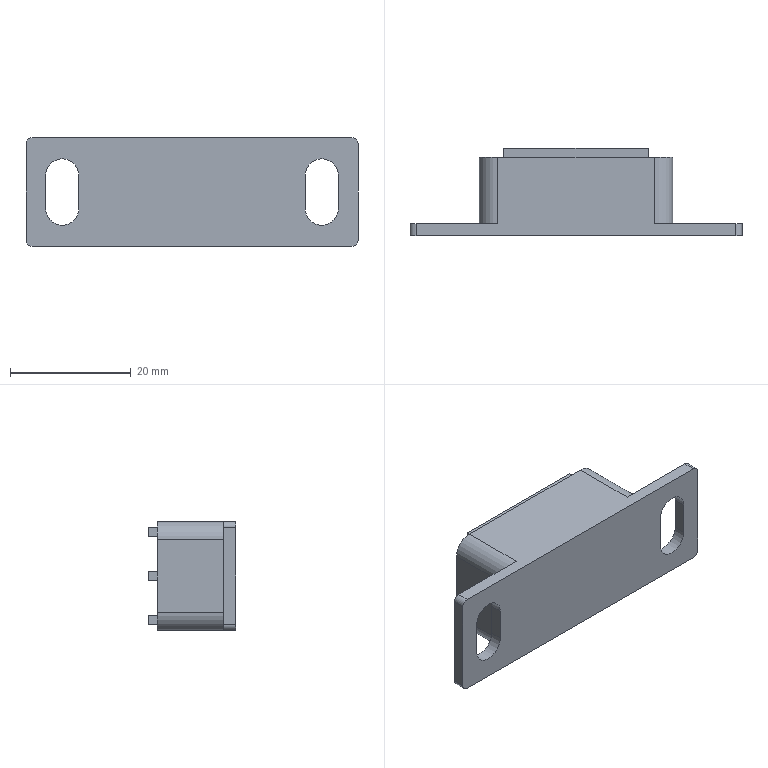Part | SolidWorks | features BaseBody 1 | 1 solid | 43 faces | box 55 x 14.5 x 18 mm | volume 8175 mm3 | plane 29 | cylinder 14 | commonest cylinder face diameters 5.5 x6 2 x4 6 x4
STEP:
#1=CARTESIAN_POINT('',(-18.75,0.,-6.25));
#2=VERTEX_POINT('',#1);
#3=CARTESIAN_POINT('',(-21.5,0.,-3.5));
#4=VERTEX_POINT('',#3);
#5=CARTESIAN_POINT('',(-21.5,0.,-6.25));
#6=DIRECTION('',(0.,-1.,0.));
#7=DIRECTION('',(0.,0.,1.));
#8=AXIS2_PLACEMENT_3D('',#5,#6,#7);
#9=CIRCLE('',#8,2.75);
#10=EDGE_CURVE('',#2,#4,#9,.T.);
#11=ORIENTED_EDGE('',*,*,#10,.T.);
#12=CARTESIAN_POINT('',(-21.5,2.,-3.5));
#13=VERTEX_POINT('',#12);
#14=CARTESIAN_POINT('',(-21.5,2.,-3.5));
#15=DIRECTION('',(0.,1.,0.));
#16=VECTOR('',#15,1000.);
#17=LINE('',#14,#16);
#18=EDGE_CURVE('',#4,#13,#17,.T.);
#19=ORIENTED_EDGE('',*,*,#18,.T.);
#20=CARTESIAN_POINT('',(-18.75,2.,-6.25));
#21=VERTEX_POINT('',#20);
#22=CARTESIAN_POINT('',(-21.5,2.,-6.25));
#23=DIRECTION('',(0.,-1.,0.));
#24=DIRECTION('',(0.,0.,1.));
#25=AXIS2_PLACEMENT_3D('',#22,#23,#24);
#26=CIRCLE('',#25,2.75);
#27=EDGE_CURVE('',#21,#13,#26,.T.);
#28=ORIENTED_EDGE('',*,*,#27,.F.);
#29=CARTESIAN_POINT('',(-18.75,2.,-6.25));
#30=DIRECTION('',(0.,1.,0.));
#31=VECTOR('',#30,1000.);
#32=LINE('',#29,#31);
#33=EDGE_CURVE('',#2,#21,#32,.T.);
#34=ORIENTED_EDGE('',*,*,#33,.F.);
#35=EDGE_LOOP('',(#11,#19,#28,#34));
#36=FACE_OUTER_BOUND('',#35,.T.);
#37=CARTESIAN_POINT('',(-21.5,2.,-6.25));
#38=DIRECTION('',(0.,1.,0.));
#39=DIRECTION('',(0.,0.,1.));
#40=AXIS2_PLACEMENT_3D('',#37,#38,#39);
#41=CYLINDRICAL_SURFACE('',#40,2.75);
#42=ADVANCED_FACE('',(#36),#41,.F.);
#43=CARTESIAN_POINT('',(24.25,0.,-6.25));
#44=VERTEX_POINT('',#43);
#45=CARTESIAN_POINT('',(21.5,0.,-3.5));
#46=VERTEX_POINT('',#45);
#47=CARTESIAN_POINT('',(21.5,0.,-6.25));
#48=DIRECTION('',(0.,-1.,0.));
#49=DIRECTION('',(0.,0.,1.));
#50=AXIS2_PLACEMENT_3D('',#47,#48,#49);
#51=CIRCLE('',#50,2.75);
#52=EDGE_CURVE('',#44,#46,#51,.T.);
#53=ORIENTED_EDGE('',*,*,#52,.T.);
#54=CARTESIAN_POINT('',(21.5,2.,-3.5));
#55=VERTEX_POINT('',#54);
#56=CARTESIAN_POINT('',(21.5,2.,-3.5));
#57=DIRECTION('',(0.,1.,0.));
#58=VECTOR('',#57,1000.);
#59=LINE('',#56,#58);
#60=EDGE_CURVE('',#46,#55,#59,.T.);
#61=ORIENTED_EDGE('',*,*,#60,.T.);
#62=CARTESIAN_POINT('',(24.25,2.,-6.25));
#63=VERTEX_POINT('',#62);
#64=CARTESIAN_POINT('',(21.5,2.,-6.25));
#65=DIRECTION('',(0.,-1.,0.));
#66=DIRECTION('',(0.,0.,1.));
#67=AXIS2_PLACEMENT_3D('',#64,#65,#66);
#68=CIRCLE('',#67,2.75);
#69=EDGE_CURVE('',#63,#55,#68,.T.);
#70=ORIENTED_EDGE('',*,*,#69,.F.);
#71=CARTESIAN_POINT('',(24.25,2.,-6.25));
#72=DIRECTION('',(0.,1.,0.));
#73=VECTOR('',#72,1000.);
#74=LINE('',#71,#73);
#75=EDGE_CURVE('',#44,#63,#74,.T.);
#76=ORIENTED_EDGE('',*,*,#75,.F.);
#77=EDGE_LOOP('',(#53,#61,#70,#76));
#78=FACE_OUTER_BOUND('',#77,.T.);
#79=CARTESIAN_POINT('',(21.5,2.,-6.25));
#80=DIRECTION('',(0.,1.,0.));
#81=DIRECTION('',(0.,0.,1.));
#82=AXIS2_PLACEMENT_3D('',#79,#80,#81);
#83=CYLINDRICAL_SURFACE('',#82,2.75);
#84=ADVANCED_FACE('',(#78),#83,.F.);
#85=ORIENTED_EDGE('',*,*,#10,.F.);
#86=CARTESIAN_POINT('',(-18.75,0.,-11.75));
#87=VERTEX_POINT('',#86);
#88=CARTESIAN_POINT('',(-18.75,0.,-1.));
#89=DIRECTION('',(0.,0.,1.));
#90=VECTOR('',#89,1000.);
#91=LINE('',#88,#90);
#92=EDGE_CURVE('',#87,#2,#91,.T.);
#93=ORIENTED_EDGE('',*,*,#92,.F.);
#94=CARTESIAN_POINT('',(-24.25,0.,-11.75));
#95=VERTEX_POINT('',#94);
#96=CARTESIAN_POINT('',(-21.5,0.,-11.75));
#97=DIRECTION('',(0.,-1.,0.));
#98=DIRECTION('',(0.,0.,1.));
#99=AXIS2_PLACEMENT_3D('',#96,#97,#98);
#100=CIRCLE('',#99,2.75);
#101=EDGE_CURVE('',#95,#87,#100,.T.);
#102=ORIENTED_EDGE('',*,*,#101,.F.);
#103=CARTESIAN_POINT('',(-24.25,0.,-6.25));
#104=VERTEX_POINT('',#103);
#105=CARTESIAN_POINT('',(-24.25,0.,-1.));
#106=DIRECTION('',(0.,0.,-1.));
#107=VECTOR('',#106,1000.);
#108=LINE('',#105,#107);
#109=EDGE_CURVE('',#104,#95,#108,.T.);
#110=ORIENTED_EDGE('',*,*,#109,.F.);
#111=CARTESIAN_POINT('',(-21.5,0.,-6.25));
#112=DIRECTION('',(0.,-1.,0.));
#113=DIRECTION('',(0.,0.,1.));
#114=AXIS2_PLACEMENT_3D('',#111,#112,#113);
#115=CIRCLE('',#114,2.75);
#116=EDGE_CURVE('',#4,#104,#115,.T.);
#117=ORIENTED_EDGE('',*,*,#116,.F.);
#118=EDGE_LOOP('',(#85,#93,#102,#110,#117));
#119=FACE_BOUND('',#118,.T.);
#120=ORIENTED_EDGE('',*,*,#52,.F.);
#121=CARTESIAN_POINT('',(24.25,0.,-11.75));
#122=VERTEX_POINT('',#121);
#123=CARTESIAN_POINT('',(24.25,0.,-1.));
#124=DIRECTION('',(0.,0.,1.));
#125=VECTOR('',#124,1000.);
#126=LINE('',#123,#125);
#127=EDGE_CURVE('',#122,#44,#126,.T.);
#128=ORIENTED_EDGE('',*,*,#127,.F.);
#129=CARTESIAN_POINT('',(18.75,0.,-11.75));
#130=VERTEX_POINT('',#129);
#131=CARTESIAN_POINT('',(21.5,0.,-11.75));
#132=DIRECTION('',(0.,-1.,0.));
#133=DIRECTION('',(0.,0.,1.));
#134=AXIS2_PLACEMENT_3D('',#131,#132,#133);
#135=CIRCLE('',#134,2.75);
#136=EDGE_CURVE('',#130,#122,#135,.T.);
#137=ORIENTED_EDGE('',*,*,#136,.F.);
#138=CARTESIAN_POINT('',(18.75,0.,-6.25));
#139=VERTEX_POINT('',#138);
#140=CARTESIAN_POINT('',(18.75,0.,-1.));
#141=DIRECTION('',(0.,0.,-1.));
#142=VECTOR('',#141,1000.);
#143=LINE('',#140,#142);
#144=EDGE_CURVE('',#139,#130,#143,.T.);
#145=ORIENTED_EDGE('',*,*,#144,.F.);
#146=CARTESIAN_POINT('',(21.5,0.,-6.25));
#147=DIRECTION('',(0.,-1.,0.));
#148=DIRECTION('',(0.,0.,1.));
#149=AXIS2_PLACEMENT_3D('',#146,#147,#148);
#150=CIRCLE('',#149,2.75);
#151=EDGE_CURVE('',#46,#139,#150,.T.);
#152=ORIENTED_EDGE('',*,*,#151,.F.);
#153=EDGE_LOOP('',(#120,#128,#137,#145,#152));
#154=FACE_BOUND('',#153,.T.);
#155=CARTESIAN_POINT('',(26.5,0.,-18.));
#156=VERTEX_POINT('',#155);
#157=CARTESIAN_POINT('',(-26.5,0.,-18.));
#158=VERTEX_POINT('',#157);
#159=CARTESIAN_POINT('',(-26.5,0.,-18.));
#160=DIRECTION('',(-1.,0.,0.));
#161=VECTOR('',#160,1000.);
#162=LINE('',#159,#161);
#163=EDGE_CURVE('',#156,#158,#162,.T.);
#164=ORIENTED_EDGE('',*,*,#163,.F.);
#165=CARTESIAN_POINT('',(27.5,0.,-17.));
#166=VERTEX_POINT('',#165);
#167=CARTESIAN_POINT('',(26.5,0.,-17.));
#168=DIRECTION('',(0.,1.,0.));
#169=DIRECTION('',(0.,0.,1.));
#170=AXIS2_PLACEMENT_3D('',#167,#168,#169);
#171=CIRCLE('',#170,1.);
#172=EDGE_CURVE('',#166,#156,#171,.T.);
#173=ORIENTED_EDGE('',*,*,#172,.F.);
#174=CARTESIAN_POINT('',(27.5,0.,-1.));
#175=VERTEX_POINT('',#174);
#176=CARTESIAN_POINT('',(27.5,0.,-1.));
#177=DIRECTION('',(0.,0.,-1.));
#178=VECTOR('',#177,1000.);
#179=LINE('',#176,#178);
#180=EDGE_CURVE('',#175,#166,#179,.T.);
#181=ORIENTED_EDGE('',*,*,#180,.F.);
#182=CARTESIAN_POINT('',(26.5,0.,0.));
#183=VERTEX_POINT('',#182);
#184=CARTESIAN_POINT('',(26.5,0.,-1.));
#185=DIRECTION('',(0.,1.,0.));
#186=DIRECTION('',(0.,0.,1.));
#187=AXIS2_PLACEMENT_3D('',#184,#185,#186);
#188=CIRCLE('',#187,1.);
#189=EDGE_CURVE('',#183,#175,#188,.T.);
#190=ORIENTED_EDGE('',*,*,#189,.F.);
#191=CARTESIAN_POINT('',(-26.5,0.,0.));
#192=VERTEX_POINT('',#191);
#193=CARTESIAN_POINT('',(-26.5,0.,0.));
#194=DIRECTION('',(1.,0.,0.));
#195=VECTOR('',#194,1000.);
#196=LINE('',#193,#195);
#197=EDGE_CURVE('',#192,#183,#196,.T.);
#198=ORIENTED_EDGE('',*,*,#197,.F.);
#199=CARTESIAN_POINT('',(-27.5,0.,-1.));
#200=VERTEX_POINT('',#199);
#201=CARTESIAN_POINT('',(-26.5,0.,-1.));
#202=DIRECTION('',(0.,1.,0.));
#203=DIRECTION('',(0.,0.,1.));
#204=AXIS2_PLACEMENT_3D('',#201,#202,#203);
#205=CIRCLE('',#204,1.);
#206=EDGE_CURVE('',#200,#192,#205,.T.);
#207=ORIENTED_EDGE('',*,*,#206,.F.);
#208=CARTESIAN_POINT('',(-27.5,0.,-17.));
#209=VERTEX_POINT('',#208);
#210=CARTESIAN_POINT('',(-27.5,0.,-1.));
#211=DIRECTION('',(0.,0.,1.));
#212=VECTOR('',#211,1000.);
#213=LINE('',#210,#212);
#214=EDGE_CURVE('',#209,#200,#213,.T.);
#215=ORIENTED_EDGE('',*,*,#214,.F.);
#216=CARTESIAN_POINT('',(-26.5,0.,-17.));
#217=DIRECTION('',(0.,1.,0.));
#218=DIRECTION('',(0.,0.,1.));
#219=AXIS2_PLACEMENT_3D('',#216,#217,#218);
#220=CIRCLE('',#219,1.);
#221=EDGE_CURVE('',#158,#209,#220,.T.);
#222=ORIENTED_EDGE('',*,*,#221,.F.);
#223=EDGE_LOOP('',(#164,#173,#181,#190,#198,#207,#215,#222));
#224=FACE_OUTER_BOUND('',#223,.T.);
#225=CARTESIAN_POINT('',(-26.5,0.,-1.));
#226=DIRECTION('',(0.,1.,0.));
#227=DIRECTION('',(0.,0.,1.));
#228=AXIS2_PLACEMENT_3D('',#225,#226,#227);
#229=PLANE('',#228);
#230=ADVANCED_FACE('',(#119,#154,#224),#229,.F.);
#231=CARTESIAN_POINT('',(-24.25,2.,-11.75));
#232=VERTEX_POINT('',#231);
#233=CARTESIAN_POINT('',(-24.25,2.,-6.25));
#234=VERTEX_POINT('',#233);
#235=CARTESIAN_POINT('',(-24.25,2.,-11.75));
#236=DIRECTION('',(0.,0.,1.));
#237=VECTOR('',#236,1000.);
#238=LINE('',#235,#237);
#239=EDGE_CURVE('',#232,#234,#238,.T.);
#240=ORIENTED_EDGE('',*,*,#239,.T.);
#241=CARTESIAN_POINT('',(-24.25,2.,-6.25));
#242=DIRECTION('',(0.,-1.,0.));
#243=VECTOR('',#242,1000.);
#244=LINE('',#241,#243);
#245=EDGE_CURVE('',#234,#104,#244,.T.);
#246=ORIENTED_EDGE('',*,*,#245,.T.);
#247=ORIENTED_EDGE('',*,*,#109,.T.);
#248=CARTESIAN_POINT('',(-24.25,2.,-11.75));
#249=DIRECTION('',(0.,1.,0.));
#250=VECTOR('',#249,1000.);
#251=LINE('',#248,#250);
#252=EDGE_CURVE('',#95,#232,#251,.T.);
#253=ORIENTED_EDGE('',*,*,#252,.T.);
#254=EDGE_LOOP('',(#240,#246,#247,#253));
#255=FACE_OUTER_BOUND('',#254,.T.);
#256=CARTESIAN_POINT('',(-24.25,2.,-11.75));
#257=DIRECTION('',(1.,0.,0.));
#258=DIRECTION('',(0.,0.,-1.));
#259=AXIS2_PLACEMENT_3D('',#256,#257,#258);
#260=PLANE('',#259);
#261=ADVANCED_FACE('',(#255),#260,.T.);
#262=ORIENTED_EDGE('',*,*,#18,.F.);
#263=ORIENTED_EDGE('',*,*,#116,.T.);
#264=ORIENTED_EDGE('',*,*,#245,.F.);
#265=CARTESIAN_POINT('',(-21.5,2.,-6.25));
#266=DIRECTION('',(0.,-1.,0.));
#267=DIRECTION('',(0.,0.,1.));
#268=AXIS2_PLACEMENT_3D('',#265,#266,#267);
#269=CIRCLE('',#268,2.75);
#270=EDGE_CURVE('',#13,#234,#269,.T.);
#271=ORIENTED_EDGE('',*,*,#270,.F.);
#272=EDGE_LOOP('',(#262,#263,#264,#271));
#273=FACE_OUTER_BOUND('',#272,.T.);
#274=CARTESIAN_POINT('',(-21.5,2.,-6.25));
#275=DIRECTION('',(0.,1.,0.));
#276=DIRECTION('',(0.,0.,1.));
#277=AXIS2_PLACEMENT_3D('',#274,#275,#276);
#278=CYLINDRICAL_SURFACE('',#277,2.75);
#279=ADVANCED_FACE('',(#273),#278,.F.);
#280=CARTESIAN_POINT('',(-18.75,2.,-11.75));
#281=VERTEX_POINT('',#280);
#282=CARTESIAN_POINT('',(-18.75,2.,-6.25));
#283=DIRECTION('',(0.,0.,-1.));
#284=VECTOR('',#283,1000.);
#285=LINE('',#282,#284);
#286=EDGE_CURVE('',#21,#281,#285,.T.);
#287=ORIENTED_EDGE('',*,*,#286,.T.);
#288=CARTESIAN_POINT('',(-18.75,2.,-11.75));
#289=DIRECTION('',(0.,-1.,0.));
#290=VECTOR('',#289,1000.);
#291=LINE('',#288,#290);
#292=EDGE_CURVE('',#281,#87,#291,.T.);
#293=ORIENTED_EDGE('',*,*,#292,.T.);
#294=ORIENTED_EDGE('',*,*,#92,.T.);
#295=ORIENTED_EDGE('',*,*,#33,.T.);
#296=EDGE_LOOP('',(#287,#293,#294,#295));
#297=FACE_OUTER_BOUND('',#296,.T.);
#298=CARTESIAN_POINT('',(-18.75,2.,-6.25));
#299=DIRECTION('',(-1.,0.,0.));
#300=DIRECTION('',(0.,0.,1.));
#301=AXIS2_PLACEMENT_3D('',#298,#299,#300);
#302=PLANE('',#301);
#303=ADVANCED_FACE('',(#297),#302,.T.);
#304=ORIENTED_EDGE('',*,*,#292,.F.);
#305=CARTESIAN_POINT('',(-21.5,2.,-11.75));
#306=DIRECTION('',(0.,-1.,0.));
#307=DIRECTION('',(0.,0.,1.));
#308=AXIS2_PLACEMENT_3D('',#305,#306,#307);
#309=CIRCLE('',#308,2.75);
#310=EDGE_CURVE('',#232,#281,#309,.T.);
#311=ORIENTED_EDGE('',*,*,#310,.F.);
#312=ORIENTED_EDGE('',*,*,#252,.F.);
#313=ORIENTED_EDGE('',*,*,#101,.T.);
#314=EDGE_LOOP('',(#304,#311,#312,#313));
#315=FACE_OUTER_BOUND('',#314,.T.);
#316=CARTESIAN_POINT('',(-21.5,2.,-11.75));
#317=DIRECTION('',(0.,1.,0.));
#318=DIRECTION('',(0.,0.,1.));
#319=AXIS2_PLACEMENT_3D('',#316,#317,#318);
#320=CYLINDRICAL_SURFACE('',#319,2.75);
#321=ADVANCED_FACE('',(#315),#320,.F.);
#322=CARTESIAN_POINT('',(18.75,2.,-11.75));
#323=VERTEX_POINT('',#322);
#324=CARTESIAN_POINT('',(18.75,2.,-6.25));
#325=VERTEX_POINT('',#324);
#326=CARTESIAN_POINT('',(18.75,2.,-11.75));
#327=DIRECTION('',(0.,0.,1.));
#328=VECTOR('',#327,1000.);
#329=LINE('',#326,#328);
#330=EDGE_CURVE('',#323,#325,#329,.T.);
#331=ORIENTED_EDGE('',*,*,#330,.T.);
#332=CARTESIAN_POINT('',(18.75,2.,-6.25));
#333=DIRECTION('',(0.,-1.,0.));
#334=VECTOR('',#333,1000.);
#335=LINE('',#332,#334);
#336=EDGE_CURVE('',#325,#139,#335,.T.);
#337=ORIENTED_EDGE('',*,*,#336,.T.);
#338=ORIENTED_EDGE('',*,*,#144,.T.);
#339=CARTESIAN_POINT('',(18.75,2.,-11.75));
#340=DIRECTION('',(0.,1.,0.));
#341=VECTOR('',#340,1000.);
#342=LINE('',#339,#341);
#343=EDGE_CURVE('',#130,#323,#342,.T.);
#344=ORIENTED_EDGE('',*,*,#343,.T.);
#345=EDGE_LOOP('',(#331,#337,#338,#344));
#346=FACE_OUTER_BOUND('',#345,.T.);
#347=CARTESIAN_POINT('',(18.75,2.,-11.75));
#348=DIRECTION('',(1.,0.,0.));
#349=DIRECTION('',(0.,0.,-1.));
#350=AXIS2_PLACEMENT_3D('',#347,#348,#349);
#351=PLANE('',#350);
#352=ADVANCED_FACE('',(#346),#351,.T.);
#353=ORIENTED_EDGE('',*,*,#60,.F.);
#354=ORIENTED_EDGE('',*,*,#151,.T.);
#355=ORIENTED_EDGE('',*,*,#336,.F.);
#356=CARTESIAN_POINT('',(21.5,2.,-6.25));
#357=DIRECTION('',(0.,-1.,0.));
#358=DIRECTION('',(0.,0.,1.));
#359=AXIS2_PLACEMENT_3D('',#356,#357,#358);
#360=CIRCLE('',#359,2.75);
#361=EDGE_CURVE('',#55,#325,#360,.T.);
#362=ORIENTED_EDGE('',*,*,#361,.F.);
#363=EDGE_LOOP('',(#353,#354,#355,#362));
#364=FACE_OUTER_BOUND('',#363,.T.);
#365=CARTESIAN_POINT('',(21.5,2.,-6.25));
#366=DIRECTION('',(0.,1.,0.));
#367=DIRECTION('',(0.,0.,1.));
#368=AXIS2_PLACEMENT_3D('',#365,#366,#367);
#369=CYLINDRICAL_SURFACE('',#368,2.75);
#370=ADVANCED_FACE('',(#364),#369,.F.);
#371=CARTESIAN_POINT('',(24.25,2.,-11.75));
#372=VERTEX_POINT('',#371);
#373=CARTESIAN_POINT('',(24.25,2.,-6.25));
#374=DIRECTION('',(0.,0.,-1.));
#375=VECTOR('',#374,1000.);
#376=LINE('',#373,#375);
#377=EDGE_CURVE('',#63,#372,#376,.T.);
#378=ORIENTED_EDGE('',*,*,#377,.T.);
#379=CARTESIAN_POINT('',(24.25,2.,-11.75));
#380=DIRECTION('',(0.,-1.,0.));
#381=VECTOR('',#380,1000.);
#382=LINE('',#379,#381);
#383=EDGE_CURVE('',#372,#122,#382,.T.);
#384=ORIENTED_EDGE('',*,*,#383,.T.);
#385=ORIENTED_EDGE('',*,*,#127,.T.);
#386=ORIENTED_EDGE('',*,*,#75,.T.);
#387=EDGE_LOOP('',(#378,#384,#385,#386));
#388=FACE_OUTER_BOUND('',#387,.T.);
#389=CARTESIAN_POINT('',(24.25,2.,-6.25));
#390=DIRECTION('',(-1.,0.,0.));
#391=DIRECTION('',(0.,0.,1.));
#392=AXIS2_PLACEMENT_3D('',#389,#390,#391);
#393=PLANE('',#392);
#394=ADVANCED_FACE('',(#388),#393,.T.);
#395=ORIENTED_EDGE('',*,*,#383,.F.);
#396=CARTESIAN_POINT('',(21.5,2.,-11.75));
#397=DIRECTION('',(0.,-1.,0.));
#398=DIRECTION('',(0.,0.,1.));
#399=AXIS2_PLACEMENT_3D('',#396,#397,#398);
#400=CIRCLE('',#399,2.75);
#401=EDGE_CURVE('',#323,#372,#400,.T.);
#402=ORIENTED_EDGE('',*,*,#401,.F.);
#403=ORIENTED_EDGE('',*,*,#343,.F.);
#404=ORIENTED_EDGE('',*,*,#136,.T.);
#405=EDGE_LOOP('',(#395,#402,#403,#404));
#406=FACE_OUTER_BOUND('',#405,.T.);
#407=CARTESIAN_POINT('',(21.5,2.,-11.75));
#408=DIRECTION('',(0.,1.,0.));
#409=DIRECTION('',(0.,0.,1.));
#410=AXIS2_PLACEMENT_3D('',#407,#408,#409);
#411=CYLINDRICAL_SURFACE('',#410,2.75);
#412=ADVANCED_FACE('',(#406),#411,.F.);
#413=CARTESIAN_POINT('',(-26.5,2.,-18.));
#414=VERTEX_POINT('',#413);
#415=CARTESIAN_POINT('',(-26.5,2.,-18.));
#416=DIRECTION('',(0.,-1.,0.));
#417=VECTOR('',#416,1000.);
#418=LINE('',#415,#417);
#419=EDGE_CURVE('',#414,#158,#418,.T.);
#420=ORIENTED_EDGE('',*,*,#419,.F.);
#421=CARTESIAN_POINT('',(-13.,2.,-18.));
#422=VERTEX_POINT('',#421);
#423=CARTESIAN_POINT('',(26.5,2.,-18.));
#424=DIRECTION('',(-1.,0.,0.));
#425=VECTOR('',#424,1000.);
#426=LINE('',#423,#425);
#427=EDGE_CURVE('',#422,#414,#426,.T.);
#428=ORIENTED_EDGE('',*,*,#427,.F.);
#429=CARTESIAN_POINT('',(-13.,13.,-18.));
#430=VERTEX_POINT('',#429);
#431=CARTESIAN_POINT('',(-13.,2.,-18.));
#432=DIRECTION('',(0.,-1.,0.));
#433=VECTOR('',#432,1000.);
#434=LINE('',#431,#433);
#435=EDGE_CURVE('',#430,#422,#434,.T.);
#436=ORIENTED_EDGE('',*,*,#435,.F.);
#437=CARTESIAN_POINT('',(13.,13.,-18.));
#438=VERTEX_POINT('',#437);
#439=CARTESIAN_POINT('',(26.5,13.,-18.));
#440=DIRECTION('',(-1.,0.,0.));
#441=VECTOR('',#440,1000.);
#442=LINE('',#439,#441);
#443=EDGE_CURVE('',#438,#430,#442,.T.);
#444=ORIENTED_EDGE('',*,*,#443,.F.);
#445=CARTESIAN_POINT('',(13.,2.,-18.));
#446=VERTEX_POINT('',#445);
#447=CARTESIAN_POINT('',(13.,2.,-18.));
#448=DIRECTION('',(0.,1.,0.));
#449=VECTOR('',#448,1000.);
#450=LINE('',#447,#449);
#451=EDGE_CURVE('',#446,#438,#450,.T.);
#452=ORIENTED_EDGE('',*,*,#451,.F.);
#453=CARTESIAN_POINT('',(26.5,2.,-18.));
#454=VERTEX_POINT('',#453);
#455=CARTESIAN_POINT('',(26.5,2.,-18.));
#456=DIRECTION('',(-1.,0.,0.));
#457=VECTOR('',#456,1000.);
#458=LINE('',#455,#457);
#459=EDGE_CURVE('',#454,#446,#458,.T.);
#460=ORIENTED_EDGE('',*,*,#459,.F.);
#461=CARTESIAN_POINT('',(26.5,2.,-18.));
#462=DIRECTION('',(0.,1.,0.));
#463=VECTOR('',#462,1000.);
#464=LINE('',#461,#463);
#465=EDGE_CURVE('',#156,#454,#464,.T.);
#466=ORIENTED_EDGE('',*,*,#465,.F.);
#467=ORIENTED_EDGE('',*,*,#163,.T.);
#468=EDGE_LOOP('',(#420,#428,#436,#444,#452,#460,#466,#467));
#469=FACE_OUTER_BOUND('',#468,.T.);
#470=CARTESIAN_POINT('',(26.5,2.,-18.));
#471=DIRECTION('',(0.,0.,1.));
#472=DIRECTION('',(1.,0.,0.));
#473=AXIS2_PLACEMENT_3D('',#470,#471,#472);
#474=PLANE('',#473);
#475=ADVANCED_FACE('',(#469),#474,.F.);
#476=CARTESIAN_POINT('',(27.5,2.,-17.));
#477=VERTEX_POINT('',#476);
#478=CARTESIAN_POINT('',(27.5,2.,-17.));
#479=DIRECTION('',(0.,-1.,0.));
#480=VECTOR('',#479,1000.);
#481=LINE('',#478,#480);
#482=EDGE_CURVE('',#477,#166,#481,.T.);
#483=ORIENTED_EDGE('',*,*,#482,.F.);
#484=CARTESIAN_POINT('',(27.5,2.,-1.));
#485=VERTEX_POINT('',#484);
#486=CARTESIAN_POINT('',(27.5,2.,-1.));
#487=DIRECTION('',(0.,0.,-1.));
#488=VECTOR('',#487,1000.);
#489=LINE('',#486,#488);
#490=EDGE_CURVE('',#485,#477,#489,.T.);
#491=ORIENTED_EDGE('',*,*,#490,.F.);
#492=CARTESIAN_POINT('',(27.5,2.,-1.));
#493=DIRECTION('',(0.,1.,0.));
#494=VECTOR('',#493,1000.);
#495=LINE('',#492,#494);
#496=EDGE_CURVE('',#175,#485,#495,.T.);
#497=ORIENTED_EDGE('',*,*,#496,.F.);
#498=ORIENTED_EDGE('',*,*,#180,.T.);
#499=EDGE_LOOP('',(#483,#491,#497,#498));
#500=FACE_OUTER_BOUND('',#499,.T.);
#501=CARTESIAN_POINT('',(27.5,2.,-1.));
#502=DIRECTION('',(-1.,0.,0.));
#503=DIRECTION('',(0.,0.,1.));
#504=AXIS2_PLACEMENT_3D('',#501,#502,#503);
#505=PLANE('',#504);
#506=ADVANCED_FACE('',(#500),#505,.F.);
#507=CARTESIAN_POINT('',(26.5,2.,0.));
#508=VERTEX_POINT('',#507);
#509=CARTESIAN_POINT('',(26.5,2.,0.));
#510=DIRECTION('',(0.,-1.,0.));
#511=VECTOR('',#510,1000.);
#512=LINE('',#509,#511);
#513=EDGE_CURVE('',#508,#183,#512,.T.);
#514=ORIENTED_EDGE('',*,*,#513,.F.);
#515=CARTESIAN_POINT('',(13.,2.,0.));
#516=VERTEX_POINT('',#515);
#517=CARTESIAN_POINT('',(-26.5,2.,0.));
#518=DIRECTION('',(1.,0.,0.));
#519=VECTOR('',#518,1000.);
#520=LINE('',#517,#519);
#521=EDGE_CURVE('',#516,#508,#520,.T.);
#522=ORIENTED_EDGE('',*,*,#521,.F.);
#523=CARTESIAN_POINT('',(13.,13.,0.));
#524=VERTEX_POINT('',#523);
#525=CARTESIAN_POINT('',(13.,2.,0.));
#526=DIRECTION('',(0.,-1.,0.));
#527=VECTOR('',#526,1000.);
#528=LINE('',#525,#527);
#529=EDGE_CURVE('',#524,#516,#528,.T.);
#530=ORIENTED_EDGE('',*,*,#529,.F.);
#531=CARTESIAN_POINT('',(-13.,13.,0.));
#532=VERTEX_POINT('',#531);
#533=CARTESIAN_POINT('',(-26.5,13.,0.));
#534=DIRECTION('',(1.,0.,0.));
#535=VECTOR('',#534,1000.);
#536=LINE('',#533,#535);
#537=EDGE_CURVE('',#532,#524,#536,.T.);
#538=ORIENTED_EDGE('',*,*,#537,.F.);
#539=CARTESIAN_POINT('',(-13.,2.,0.));
#540=VERTEX_POINT('',#539);
#541=CARTESIAN_POINT('',(-13.,2.,0.));
#542=DIRECTION('',(0.,1.,0.));
#543=VECTOR('',#542,1000.);
#544=LINE('',#541,#543);
#545=EDGE_CURVE('',#540,#532,#544,.T.);
#546=ORIENTED_EDGE('',*,*,#545,.F.);
#547=CARTESIAN_POINT('',(-26.5,2.,0.));
#548=VERTEX_POINT('',#547);
#549=CARTESIAN_POINT('',(-26.5,2.,0.));
#550=DIRECTION('',(1.,0.,0.));
#551=VECTOR('',#550,1000.);
#552=LINE('',#549,#551);
#553=EDGE_CURVE('',#548,#540,#552,.T.);
#554=ORIENTED_EDGE('',*,*,#553,.F.);
#555=CARTESIAN_POINT('',(-26.5,2.,0.));
#556=DIRECTION('',(0.,1.,0.));
#557=VECTOR('',#556,1000.);
#558=LINE('',#555,#557);
#559=EDGE_CURVE('',#192,#548,#558,.T.);
#560=ORIENTED_EDGE('',*,*,#559,.F.);
#561=ORIENTED_EDGE('',*,*,#197,.T.);
#562=EDGE_LOOP('',(#514,#522,#530,#538,#546,#554,#560,#561));
#563=FACE_OUTER_BOUND('',#562,.T.);
#564=CARTESIAN_POINT('',(-26.5,2.,0.));
#565=DIRECTION('',(0.,0.,-1.));
#566=DIRECTION('',(-1.,0.,0.));
#567=AXIS2_PLACEMENT_3D('',#564,#565,#566);
#568=PLANE('',#567);
#569=ADVANCED_FACE('',(#563),#568,.F.);
#570=CARTESIAN_POINT('',(-27.5,2.,-1.));
#571=VERTEX_POINT('',#570);
#572=CARTESIAN_POINT('',(-27.5,2.,-1.));
#573=DIRECTION('',(0.,-1.,0.));
#574=VECTOR('',#573,1000.);
#575=LINE('',#572,#574);
#576=EDGE_CURVE('',#571,#200,#575,.T.);
#577=ORIENTED_EDGE('',*,*,#576,.F.);
#578=CARTESIAN_POINT('',(-27.5,2.,-17.));
#579=VERTEX_POINT('',#578);
#580=CARTESIAN_POINT('',(-27.5,2.,-17.));
#581=DIRECTION('',(0.,0.,1.));
#582=VECTOR('',#581,1000.);
#583=LINE('',#580,#582);
#584=EDGE_CURVE('',#579,#571,#583,.T.);
#585=ORIENTED_EDGE('',*,*,#584,.F.);
#586=CARTESIAN_POINT('',(-27.5,2.,-17.));
#587=DIRECTION('',(0.,1.,0.));
#588=VECTOR('',#587,1000.);
#589=LINE('',#586,#588);
#590=EDGE_CURVE('',#209,#579,#589,.T.);
#591=ORIENTED_EDGE('',*,*,#590,.F.);
#592=ORIENTED_EDGE('',*,*,#214,.T.);
#593=EDGE_LOOP('',(#577,#585,#591,#592));
#594=FACE_OUTER_BOUND('',#593,.T.);
#595=CARTESIAN_POINT('',(-27.5,2.,-17.));
#596=DIRECTION('',(1.,0.,0.));
#597=DIRECTION('',(0.,0.,-1.));
#598=AXIS2_PLACEMENT_3D('',#595,#596,#597);
#599=PLANE('',#598);
#600=ADVANCED_FACE('',(#594),#599,.F.);
#601=ORIENTED_EDGE('',*,*,#553,.T.);
#602=CARTESIAN_POINT('',(-16.,2.,-3.));
#603=VERTEX_POINT('',#602);
#604=CARTESIAN_POINT('',(-13.,2.,-3.));
#605=DIRECTION('',(0.,-1.,0.));
#606=DIRECTION('',(0.,0.,1.));
#607=AXIS2_PLACEMENT_3D('',#604,#605,#606);
#608=CIRCLE('',#607,3.);
#609=EDGE_CURVE('',#540,#603,#608,.T.);
#610=ORIENTED_EDGE('',*,*,#609,.T.);
#611=CARTESIAN_POINT('',(-16.,2.,-15.));
#612=VERTEX_POINT('',#611);
#613=CARTESIAN_POINT('',(-16.,2.,-1.));
#614=DIRECTION('',(0.,0.,-1.));
#615=VECTOR('',#614,1000.);
#616=LINE('',#613,#615);
#617=EDGE_CURVE('',#603,#612,#616,.T.);
#618=ORIENTED_EDGE('',*,*,#617,.T.);
#619=CARTESIAN_POINT('',(-13.,2.,-15.));
#620=DIRECTION('',(0.,-1.,0.));
#621=DIRECTION('',(0.,0.,1.));
#622=AXIS2_PLACEMENT_3D('',#619,#620,#621);
#623=CIRCLE('',#622,3.);
#624=EDGE_CURVE('',#612,#422,#623,.T.);
#625=ORIENTED_EDGE('',*,*,#624,.T.);
#626=ORIENTED_EDGE('',*,*,#427,.T.);
#627=CARTESIAN_POINT('',(-26.5,2.,-17.));
#628=DIRECTION('',(0.,1.,0.));
#629=DIRECTION('',(0.,0.,1.));
#630=AXIS2_PLACEMENT_3D('',#627,#628,#629);
#631=CIRCLE('',#630,1.);
#632=EDGE_CURVE('',#414,#579,#631,.T.);
#633=ORIENTED_EDGE('',*,*,#632,.T.);
#634=ORIENTED_EDGE('',*,*,#584,.T.);
#635=CARTESIAN_POINT('',(-26.5,2.,-1.));
#636=DIRECTION('',(0.,1.,0.));
#637=DIRECTION('',(0.,0.,1.));
#638=AXIS2_PLACEMENT_3D('',#635,#636,#637);
#639=CIRCLE('',#638,1.);
#640=EDGE_CURVE('',#571,#548,#639,.T.);
#641=ORIENTED_EDGE('',*,*,#640,.T.);
#642=EDGE_LOOP('',(#601,#610,#618,#625,#626,#633,#634,#641));
#643=FACE_OUTER_BOUND('',#642,.T.);
#644=ORIENTED_EDGE('',*,*,#286,.F.);
#645=ORIENTED_EDGE('',*,*,#27,.T.);
#646=ORIENTED_EDGE('',*,*,#270,.T.);
#647=ORIENTED_EDGE('',*,*,#239,.F.);
#648=ORIENTED_EDGE('',*,*,#310,.T.);
#649=EDGE_LOOP('',(#644,#645,#646,#647,#648));
#650=FACE_BOUND('',#649,.T.);
#651=CARTESIAN_POINT('',(-26.5,2.,-1.));
#652=DIRECTION('',(0.,1.,0.));
#653=DIRECTION('',(0.,0.,1.));
#654=AXIS2_PLACEMENT_3D('',#651,#652,#653);
#655=PLANE('',#654);
#656=ADVANCED_FACE('',(#643,#650),#655,.T.);
#657=ORIENTED_EDGE('',*,*,#459,.T.);
#658=CARTESIAN_POINT('',(16.,2.,-15.));
#659=VERTEX_POINT('',#658);
#660=CARTESIAN_POINT('',(13.,2.,-15.));
#661=DIRECTION('',(0.,-1.,0.));
#662=DIRECTION('',(0.,0.,1.));
#663=AXIS2_PLACEMENT_3D('',#660,#661,#662);
#664=CIRCLE('',#663,3.);
#665=EDGE_CURVE('',#446,#659,#664,.T.);
#666=ORIENTED_EDGE('',*,*,#665,.T.);
#667=CARTESIAN_POINT('',(16.,2.,-3.));
#668=VERTEX_POINT('',#667);
#669=CARTESIAN_POINT('',(16.,2.,-1.));
#670=DIRECTION('',(0.,0.,1.));
#671=VECTOR('',#670,1000.);
#672=LINE('',#669,#671);
#673=EDGE_CURVE('',#659,#668,#672,.T.);
#674=ORIENTED_EDGE('',*,*,#673,.T.);
#675=CARTESIAN_POINT('',(13.,2.,-3.));
#676=DIRECTION('',(0.,-1.,0.));
#677=DIRECTION('',(0.,0.,1.));
#678=AXIS2_PLACEMENT_3D('',#675,#676,#677);
#679=CIRCLE('',#678,3.);
#680=EDGE_CURVE('',#668,#516,#679,.T.);
#681=ORIENTED_EDGE('',*,*,#680,.T.);
#682=ORIENTED_EDGE('',*,*,#521,.T.);
#683=CARTESIAN_POINT('',(26.5,2.,-1.));
#684=DIRECTION('',(0.,1.,0.));
#685=DIRECTION('',(0.,0.,1.));
#686=AXIS2_PLACEMENT_3D('',#683,#684,#685);
#687=CIRCLE('',#686,1.);
#688=EDGE_CURVE('',#508,#485,#687,.T.);
#689=ORIENTED_EDGE('',*,*,#688,.T.);
#690=ORIENTED_EDGE('',*,*,#490,.T.);
#691=CARTESIAN_POINT('',(26.5,2.,-17.));
#692=DIRECTION('',(0.,1.,0.));
#693=DIRECTION('',(0.,0.,1.));
#694=AXIS2_PLACEMENT_3D('',#691,#692,#693);
#695=CIRCLE('',#694,1.);
#696=EDGE_CURVE('',#477,#454,#695,.T.);
#697=ORIENTED_EDGE('',*,*,#696,.T.);
#698=EDGE_LOOP('',(#657,#666,#674,#681,#682,#689,#690,#697));
#699=FACE_OUTER_BOUND('',#698,.T.);
#700=ORIENTED_EDGE('',*,*,#377,.F.);
#701=ORIENTED_EDGE('',*,*,#69,.T.);
#702=ORIENTED_EDGE('',*,*,#361,.T.);
#703=ORIENTED_EDGE('',*,*,#330,.F.);
#704=ORIENTED_EDGE('',*,*,#401,.T.);
#705=EDGE_LOOP('',(#700,#701,#702,#703,#704));
#706=FACE_BOUND('',#705,.T.);
#707=CARTESIAN_POINT('',(-26.5,2.,-1.));
#708=DIRECTION('',(0.,1.,0.));
#709=DIRECTION('',(0.,0.,1.));
#710=AXIS2_PLACEMENT_3D('',#707,#708,#709);
#711=PLANE('',#710);
#712=ADVANCED_FACE('',(#699,#706),#711,.T.);
#713=ORIENTED_EDGE('',*,*,#632,.F.);
#714=ORIENTED_EDGE('',*,*,#419,.T.);
#715=ORIENTED_EDGE('',*,*,#221,.T.);
#716=ORIENTED_EDGE('',*,*,#590,.T.);
#717=EDGE_LOOP('',(#713,#714,#715,#716));
#718=FACE_OUTER_BOUND('',#717,.T.);
#719=CARTESIAN_POINT('',(-26.5,2.,-17.));
#720=DIRECTION('',(0.,1.,0.));
#721=DIRECTION('',(0.,0.,1.));
#722=AXIS2_PLACEMENT_3D('',#719,#720,#721);
#723=CYLINDRICAL_SURFACE('',#722,1.);
#724=ADVANCED_FACE('',(#718),#723,.T.);
#725=CARTESIAN_POINT('',(-16.,13.,-15.));
#726=VERTEX_POINT('',#725);
#727=CARTESIAN_POINT('',(-13.,13.,-15.));
#728=DIRECTION('',(0.,-1.,0.));
#729=DIRECTION('',(0.,0.,1.));
#730=AXIS2_PLACEMENT_3D('',#727,#728,#729);
#731=CIRCLE('',#730,3.);
#732=EDGE_CURVE('',#726,#430,#731,.T.);
#733=ORIENTED_EDGE('',*,*,#732,.T.);
#734=ORIENTED_EDGE('',*,*,#435,.T.);
#735=ORIENTED_EDGE('',*,*,#624,.F.);
#736=CARTESIAN_POINT('',(-16.,13.,-15.));
#737=DIRECTION('',(0.,1.,0.));
#738=VECTOR('',#737,1000.);
#739=LINE('',#736,#738);
#740=EDGE_CURVE('',#612,#726,#739,.T.);
#741=ORIENTED_EDGE('',*,*,#740,.T.);
#742=EDGE_LOOP('',(#733,#734,#735,#741));
#743=FACE_OUTER_BOUND('',#742,.T.);
#744=CARTESIAN_POINT('',(-13.,13.,-15.));
#745=DIRECTION('',(0.,1.,0.));
#746=DIRECTION('',(0.,0.,1.));
#747=AXIS2_PLACEMENT_3D('',#744,#745,#746);
#748=CYLINDRICAL_SURFACE('',#747,3.);
#749=ADVANCED_FACE('',(#743),#748,.T.);
#750=CARTESIAN_POINT('',(-12.,13.,-17.));
#751=VERTEX_POINT('',#750);
#752=CARTESIAN_POINT('',(12.,13.,-17.));
#753=VERTEX_POINT('',#752);
#754=CARTESIAN_POINT('',(-13.,13.,-17.));
#755=DIRECTION('',(1.,0.,0.));
#756=VECTOR('',#755,1000.);
#757=LINE('',#754,#756);
#758=EDGE_CURVE('',#751,#753,#757,.T.);
#759=ORIENTED_EDGE('',*,*,#758,.T.);
#760=CARTESIAN_POINT('',(12.,13.,-15.5));
#761=VERTEX_POINT('',#760);
#762=CARTESIAN_POINT('',(12.,13.,-15.));
#763=DIRECTION('',(0.,0.,1.));
#764=VECTOR('',#763,1000.);
#765=LINE('',#762,#764);
#766=EDGE_CURVE('',#753,#761,#765,.T.);
#767=ORIENTED_EDGE('',*,*,#766,.T.);
#768=CARTESIAN_POINT('',(-12.,13.,-15.5));
#769=VERTEX_POINT('',#768);
#770=CARTESIAN_POINT('',(-13.,13.,-15.5));
#771=DIRECTION('',(-1.,0.,0.));
#772=VECTOR('',#771,1000.);
#773=LINE('',#770,#772);
#774=EDGE_CURVE('',#761,#769,#773,.T.);
#775=ORIENTED_EDGE('',*,*,#774,.T.);
#776=CARTESIAN_POINT('',(-12.,13.,-15.));
#777=DIRECTION('',(0.,0.,-1.));
#778=VECTOR('',#777,1000.);
#779=LINE('',#776,#778);
#780=EDGE_CURVE('',#769,#751,#779,.T.);
#781=ORIENTED_EDGE('',*,*,#780,.T.);
#782=EDGE_LOOP('',(#759,#767,#775,#781));
#783=FACE_BOUND('',#782,.T.);
#784=CARTESIAN_POINT('',(-12.,13.,-9.75));
#785=VERTEX_POINT('',#784);
#786=CARTESIAN_POINT('',(12.,13.,-9.75));
#787=VERTEX_POINT('',#786);
#788=CARTESIAN_POINT('',(-13.,13.,-9.75));
#789=DIRECTION('',(1.,0.,0.));
#790=VECTOR('',#789,1000.);
#791=LINE('',#788,#790);
#792=EDGE_CURVE('',#785,#787,#791,.T.);
#793=ORIENTED_EDGE('',*,*,#792,.T.);
#794=CARTESIAN_POINT('',(12.,13.,-8.25));
#795=VERTEX_POINT('',#794);
#796=CARTESIAN_POINT('',(12.,13.,-15.));
#797=DIRECTION('',(0.,0.,1.));
#798=VECTOR('',#797,1000.);
#799=LINE('',#796,#798);
#800=EDGE_CURVE('',#787,#795,#799,.T.);
#801=ORIENTED_EDGE('',*,*,#800,.T.);
#802=CARTESIAN_POINT('',(-12.,13.,-8.25));
#803=VERTEX_POINT('',#802);
#804=CARTESIAN_POINT('',(-13.,13.,-8.25));
#805=DIRECTION('',(-1.,0.,0.));
#806=VECTOR('',#805,1000.);
#807=LINE('',#804,#806);
#808=EDGE_CURVE('',#795,#803,#807,.T.);
#809=ORIENTED_EDGE('',*,*,#808,.T.);
#810=CARTESIAN_POINT('',(-12.,13.,-15.));
#811=DIRECTION('',(0.,0.,-1.));
#812=VECTOR('',#811,1000.);
#813=LINE('',#810,#812);
#814=EDGE_CURVE('',#803,#785,#813,.T.);
#815=ORIENTED_EDGE('',*,*,#814,.T.);
#816=EDGE_LOOP('',(#793,#801,#809,#815));
#817=FACE_BOUND('',#816,.T.);
#818=CARTESIAN_POINT('',(-12.,13.,-2.5));
#819=VERTEX_POINT('',#818);
#820=CARTESIAN_POINT('',(12.,13.,-2.5));
#821=VERTEX_POINT('',#820);
#822=CARTESIAN_POINT('',(-13.,13.,-2.5));
#823=DIRECTION('',(1.,0.,0.));
#824=VECTOR('',#823,1000.);
#825=LINE('',#822,#824);
#826=EDGE_CURVE('',#819,#821,#825,.T.);
#827=ORIENTED_EDGE('',*,*,#826,.T.);
#828=CARTESIAN_POINT('',(12.,13.,-1.));
#829=VERTEX_POINT('',#828);
#830=CARTESIAN_POINT('',(12.,13.,-15.));
#831=DIRECTION('',(0.,0.,1.));
#832=VECTOR('',#831,1000.);
#833=LINE('',#830,#832);
#834=EDGE_CURVE('',#821,#829,#833,.T.);
#835=ORIENTED_EDGE('',*,*,#834,.T.);
#836=CARTESIAN_POINT('',(-12.,13.,-1.));
#837=VERTEX_POINT('',#836);
#838=CARTESIAN_POINT('',(-13.,13.,-1.));
#839=DIRECTION('',(-1.,0.,0.));
#840=VECTOR('',#839,1000.);
#841=LINE('',#838,#840);
#842=EDGE_CURVE('',#829,#837,#841,.T.);
#843=ORIENTED_EDGE('',*,*,#842,.T.);
#844=CARTESIAN_POINT('',(-12.,13.,-15.));
#845=DIRECTION('',(0.,0.,-1.));
#846=VECTOR('',#845,1000.);
#847=LINE('',#844,#846);
#848=EDGE_CURVE('',#837,#819,#847,.T.);
#849=ORIENTED_EDGE('',*,*,#848,.T.);
#850=EDGE_LOOP('',(#827,#835,#843,#849));
#851=FACE_BOUND('',#850,.T.);
#852=CARTESIAN_POINT('',(16.,13.,-15.));
#853=VERTEX_POINT('',#852);
#854=CARTESIAN_POINT('',(13.,13.,-15.));
#855=DIRECTION('',(0.,1.,0.));
#856=DIRECTION('',(0.,0.,1.));
#857=AXIS2_PLACEMENT_3D('',#854,#855,#856);
#858=CIRCLE('',#857,3.);
#859=EDGE_CURVE('',#853,#438,#858,.T.);
#860=ORIENTED_EDGE('',*,*,#859,.T.);
#861=ORIENTED_EDGE('',*,*,#443,.T.);
#862=ORIENTED_EDGE('',*,*,#732,.F.);
#863=CARTESIAN_POINT('',(-16.,13.,-3.));
#864=VERTEX_POINT('',#863);
#865=CARTESIAN_POINT('',(-16.,13.,-15.));
#866=DIRECTION('',(0.,0.,1.));
#867=VECTOR('',#866,1000.);
#868=LINE('',#865,#867);
#869=EDGE_CURVE('',#726,#864,#868,.T.);
#870=ORIENTED_EDGE('',*,*,#869,.T.);
#871=CARTESIAN_POINT('',(-13.,13.,-3.));
#872=DIRECTION('',(0.,1.,0.));
#873=DIRECTION('',(0.,0.,1.));
#874=AXIS2_PLACEMENT_3D('',#871,#872,#873);
#875=CIRCLE('',#874,3.);
#876=EDGE_CURVE('',#864,#532,#875,.T.);
#877=ORIENTED_EDGE('',*,*,#876,.T.);
#878=ORIENTED_EDGE('',*,*,#537,.T.);
#879=CARTESIAN_POINT('',(16.,13.,-3.));
#880=VERTEX_POINT('',#879);
#881=CARTESIAN_POINT('',(13.,13.,-3.));
#882=DIRECTION('',(0.,1.,0.));
#883=DIRECTION('',(0.,0.,1.));
#884=AXIS2_PLACEMENT_3D('',#881,#882,#883);
#885=CIRCLE('',#884,3.);
#886=EDGE_CURVE('',#524,#880,#885,.T.);
#887=ORIENTED_EDGE('',*,*,#886,.T.);
#888=CARTESIAN_POINT('',(16.,13.,-15.));
#889=DIRECTION('',(0.,0.,-1.));
#890=VECTOR('',#889,1000.);
#891=LINE('',#888,#890);
#892=EDGE_CURVE('',#880,#853,#891,.T.);
#893=ORIENTED_EDGE('',*,*,#892,.T.);
#894=EDGE_LOOP('',(#860,#861,#862,#870,#877,#878,#887,#893));
#895=FACE_OUTER_BOUND('',#894,.T.);
#896=CARTESIAN_POINT('',(-13.,13.,-15.));
#897=DIRECTION('',(0.,1.,0.));
#898=DIRECTION('',(0.,0.,1.));
#899=AXIS2_PLACEMENT_3D('',#896,#897,#898);
#900=PLANE('',#899);
#901=ADVANCED_FACE('',(#783,#817,#851,#895),#900,.T.);
#902=ORIENTED_EDGE('',*,*,#859,.F.);
#903=CARTESIAN_POINT('',(16.,13.,-15.));
#904=DIRECTION('',(0.,-1.,0.));
#905=VECTOR('',#904,1000.);
#906=LINE('',#903,#905);
#907=EDGE_CURVE('',#853,#659,#906,.T.);
#908=ORIENTED_EDGE('',*,*,#907,.T.);
#909=ORIENTED_EDGE('',*,*,#665,.F.);
#910=ORIENTED_EDGE('',*,*,#451,.T.);
#911=EDGE_LOOP('',(#902,#908,#909,#910));
#912=FACE_OUTER_BOUND('',#911,.T.);
#913=CARTESIAN_POINT('',(13.,13.,-15.));
#914=DIRECTION('',(0.,1.,0.));
#915=DIRECTION('',(0.,0.,1.));
#916=AXIS2_PLACEMENT_3D('',#913,#914,#915);
#917=CYLINDRICAL_SURFACE('',#916,3.);
#918=ADVANCED_FACE('',(#912),#917,.T.);
#919=ORIENTED_EDGE('',*,*,#696,.F.);
#920=ORIENTED_EDGE('',*,*,#482,.T.);
#921=ORIENTED_EDGE('',*,*,#172,.T.);
#922=ORIENTED_EDGE('',*,*,#465,.T.);
#923=EDGE_LOOP('',(#919,#920,#921,#922));
#924=FACE_OUTER_BOUND('',#923,.T.);
#925=CARTESIAN_POINT('',(26.5,2.,-17.));
#926=DIRECTION('',(0.,1.,0.));
#927=DIRECTION('',(0.,0.,1.));
#928=AXIS2_PLACEMENT_3D('',#925,#926,#927);
#929=CYLINDRICAL_SURFACE('',#928,1.);
#930=ADVANCED_FACE('',(#924),#929,.T.);
#931=ORIENTED_EDGE('',*,*,#688,.F.);
#932=ORIENTED_EDGE('',*,*,#513,.T.);
#933=ORIENTED_EDGE('',*,*,#189,.T.);
#934=ORIENTED_EDGE('',*,*,#496,.T.);
#935=EDGE_LOOP('',(#931,#932,#933,#934));
#936=FACE_OUTER_BOUND('',#935,.T.);
#937=CARTESIAN_POINT('',(26.5,2.,-1.));
#938=DIRECTION('',(0.,1.,0.));
#939=DIRECTION('',(0.,0.,1.));
#940=AXIS2_PLACEMENT_3D('',#937,#938,#939);
#941=CYLINDRICAL_SURFACE('',#940,1.);
#942=ADVANCED_FACE('',(#936),#941,.T.);
#943=ORIENTED_EDGE('',*,*,#886,.F.);
#944=ORIENTED_EDGE('',*,*,#529,.T.);
#945=ORIENTED_EDGE('',*,*,#680,.F.);
#946=CARTESIAN_POINT('',(16.,13.,-3.));
#947=DIRECTION('',(0.,1.,0.));
#948=VECTOR('',#947,1000.);
#949=LINE('',#946,#948);
#950=EDGE_CURVE('',#668,#880,#949,.T.);
#951=ORIENTED_EDGE('',*,*,#950,.T.);
#952=EDGE_LOOP('',(#943,#944,#945,#951));
#953=FACE_OUTER_BOUND('',#952,.T.);
#954=CARTESIAN_POINT('',(13.,13.,-3.));
#955=DIRECTION('',(0.,1.,0.));
#956=DIRECTION('',(0.,0.,1.));
#957=AXIS2_PLACEMENT_3D('',#954,#955,#956);
#958=CYLINDRICAL_SURFACE('',#957,3.);
#959=ADVANCED_FACE('',(#953),#958,.T.);
#960=ORIENTED_EDGE('',*,*,#876,.F.);
#961=CARTESIAN_POINT('',(-16.,13.,-3.));
#962=DIRECTION('',(0.,-1.,0.));
#963=VECTOR('',#962,1000.);
#964=LINE('',#961,#963);
#965=EDGE_CURVE('',#864,#603,#964,.T.);
#966=ORIENTED_EDGE('',*,*,#965,.T.);
#967=ORIENTED_EDGE('',*,*,#609,.F.);
#968=ORIENTED_EDGE('',*,*,#545,.T.);
#969=EDGE_LOOP('',(#960,#966,#967,#968));
#970=FACE_OUTER_BOUND('',#969,.T.);
#971=CARTESIAN_POINT('',(-13.,13.,-3.));
#972=DIRECTION('',(0.,1.,0.));
#973=DIRECTION('',(0.,0.,1.));
#974=AXIS2_PLACEMENT_3D('',#971,#972,#973);
#975=CYLINDRICAL_SURFACE('',#974,3.);
#976=ADVANCED_FACE('',(#970),#975,.T.);
#977=ORIENTED_EDGE('',*,*,#640,.F.);
#978=ORIENTED_EDGE('',*,*,#576,.T.);
#979=ORIENTED_EDGE('',*,*,#206,.T.);
#980=ORIENTED_EDGE('',*,*,#559,.T.);
#981=EDGE_LOOP('',(#977,#978,#979,#980));
#982=FACE_OUTER_BOUND('',#981,.T.);
#983=CARTESIAN_POINT('',(-26.5,2.,-1.));
#984=DIRECTION('',(0.,1.,0.));
#985=DIRECTION('',(0.,0.,1.));
#986=AXIS2_PLACEMENT_3D('',#983,#984,#985);
#987=CYLINDRICAL_SURFACE('',#986,1.);
#988=ADVANCED_FACE('',(#982),#987,.T.);
#989=ORIENTED_EDGE('',*,*,#965,.F.);
#990=ORIENTED_EDGE('',*,*,#869,.F.);
#991=ORIENTED_EDGE('',*,*,#740,.F.);
#992=ORIENTED_EDGE('',*,*,#617,.F.);
#993=EDGE_LOOP('',(#989,#990,#991,#992));
#994=FACE_OUTER_BOUND('',#993,.T.);
#995=CARTESIAN_POINT('',(-16.,13.,-15.));
#996=DIRECTION('',(1.,0.,0.));
#997=DIRECTION('',(0.,0.,-1.));
#998=AXIS2_PLACEMENT_3D('',#995,#996,#997);
#999=PLANE('',#998);
#1000=ADVANCED_FACE('',(#994),#999,.F.);
#1001=ORIENTED_EDGE('',*,*,#907,.F.);
#1002=ORIENTED_EDGE('',*,*,#892,.F.);
#1003=ORIENTED_EDGE('',*,*,#950,.F.);
#1004=ORIENTED_EDGE('',*,*,#673,.F.);
#1005=EDGE_LOOP('',(#1001,#1002,#1003,#1004));
#1006=FACE_OUTER_BOUND('',#1005,.T.);
#1007=CARTESIAN_POINT('',(16.,13.,-3.));
#1008=DIRECTION('',(-1.,0.,0.));
#1009=DIRECTION('',(0.,0.,1.));
#1010=AXIS2_PLACEMENT_3D('',#1007,#1008,#1009);
#1011=PLANE('',#1010);
#1012=ADVANCED_FACE('',(#1006),#1011,.F.);
#1013=CARTESIAN_POINT('',(12.,14.5,-17.));
#1014=VERTEX_POINT('',#1013);
#1015=CARTESIAN_POINT('',(12.,14.5,-17.));
#1016=DIRECTION('',(0.,-1.,0.));
#1017=VECTOR('',#1016,1000.);
#1018=LINE('',#1015,#1017);
#1019=EDGE_CURVE('',#1014,#753,#1018,.T.);
#1020=ORIENTED_EDGE('',*,*,#1019,.F.);
#1021=CARTESIAN_POINT('',(12.,14.5,-15.5));
#1022=VERTEX_POINT('',#1021);
#1023=CARTESIAN_POINT('',(12.,14.5,0.));
#1024=DIRECTION('',(0.,0.,-1.));
#1025=VECTOR('',#1024,1000.);
#1026=LINE('',#1023,#1025);
#1027=EDGE_CURVE('',#1022,#1014,#1026,.T.);
#1028=ORIENTED_EDGE('',*,*,#1027,.F.);
#1029=CARTESIAN_POINT('',(12.,14.5,-15.5));
#1030=DIRECTION('',(0.,1.,0.));
#1031=VECTOR('',#1030,1000.);
#1032=LINE('',#1029,#1031);
#1033=EDGE_CURVE('',#761,#1022,#1032,.T.);
#1034=ORIENTED_EDGE('',*,*,#1033,.F.);
#1035=ORIENTED_EDGE('',*,*,#766,.F.);
#1036=EDGE_LOOP('',(#1020,#1028,#1034,#1035));
#1037=FACE_OUTER_BOUND('',#1036,.T.);
#1038=CARTESIAN_POINT('',(12.,14.5,-15.5));
#1039=DIRECTION('',(-1.,0.,0.));
#1040=DIRECTION('',(0.,0.,1.));
#1041=AXIS2_PLACEMENT_3D('',#1038,#1039,#1040);
#1042=PLANE('',#1041);
#1043=ADVANCED_FACE('',(#1037),#1042,.F.);
#1044=CARTESIAN_POINT('',(-12.,14.5,-17.));
#1045=VERTEX_POINT('',#1044);
#1046=CARTESIAN_POINT('',(-12.,14.5,-17.));
#1047=DIRECTION('',(0.,-1.,0.));
#1048=VECTOR('',#1047,1000.);
#1049=LINE('',#1046,#1048);
#1050=EDGE_CURVE('',#1045,#751,#1049,.T.);
#1051=ORIENTED_EDGE('',*,*,#1050,.F.);
#1052=CARTESIAN_POINT('',(12.,14.5,-17.));
#1053=DIRECTION('',(-1.,0.,0.));
#1054=VECTOR('',#1053,1000.);
#1055=LINE('',#1052,#1054);
#1056=EDGE_CURVE('',#1014,#1045,#1055,.T.);
#1057=ORIENTED_EDGE('',*,*,#1056,.F.);
#1058=ORIENTED_EDGE('',*,*,#1019,.T.);
#1059=ORIENTED_EDGE('',*,*,#758,.F.);
#1060=EDGE_LOOP('',(#1051,#1057,#1058,#1059));
#1061=FACE_OUTER_BOUND('',#1060,.T.);
#1062=CARTESIAN_POINT('',(12.,14.5,-17.));
#1063=DIRECTION('',(0.,0.,1.));
#1064=DIRECTION('',(1.,0.,0.));
#1065=AXIS2_PLACEMENT_3D('',#1062,#1063,#1064);
#1066=PLANE('',#1065);
#1067=ADVANCED_FACE('',(#1061),#1066,.F.);
#1068=CARTESIAN_POINT('',(-12.,14.5,-15.5));
#1069=VERTEX_POINT('',#1068);
#1070=CARTESIAN_POINT('',(-12.,14.5,-15.5));
#1071=DIRECTION('',(0.,-1.,0.));
#1072=VECTOR('',#1071,1000.);
#1073=LINE('',#1070,#1072);
#1074=EDGE_CURVE('',#1069,#769,#1073,.T.);
#1075=ORIENTED_EDGE('',*,*,#1074,.F.);
#1076=CARTESIAN_POINT('',(-12.,14.5,-17.));
#1077=DIRECTION('',(0.,0.,1.));
#1078=VECTOR('',#1077,1000.);
#1079=LINE('',#1076,#1078);
#1080=EDGE_CURVE('',#1045,#1069,#1079,.T.);
#1081=ORIENTED_EDGE('',*,*,#1080,.F.);
#1082=ORIENTED_EDGE('',*,*,#1050,.T.);
#1083=ORIENTED_EDGE('',*,*,#780,.F.);
#1084=EDGE_LOOP('',(#1075,#1081,#1082,#1083));
#1085=FACE_OUTER_BOUND('',#1084,.T.);
#1086=CARTESIAN_POINT('',(-12.,14.5,-17.));
#1087=DIRECTION('',(1.,0.,0.));
#1088=DIRECTION('',(0.,0.,-1.));
#1089=AXIS2_PLACEMENT_3D('',#1086,#1087,#1088);
#1090=PLANE('',#1089);
#1091=ADVANCED_FACE('',(#1085),#1090,.F.);
#1092=ORIENTED_EDGE('',*,*,#1033,.T.);
#1093=CARTESIAN_POINT('',(-12.,14.5,-15.5));
#1094=DIRECTION('',(1.,0.,0.));
#1095=VECTOR('',#1094,1000.);
#1096=LINE('',#1093,#1095);
#1097=EDGE_CURVE('',#1069,#1022,#1096,.T.);
#1098=ORIENTED_EDGE('',*,*,#1097,.F.);
#1099=ORIENTED_EDGE('',*,*,#1074,.T.);
#1100=ORIENTED_EDGE('',*,*,#774,.F.);
#1101=EDGE_LOOP('',(#1092,#1098,#1099,#1100));
#1102=FACE_OUTER_BOUND('',#1101,.T.);
#1103=CARTESIAN_POINT('',(-12.,14.5,-15.5));
#1104=DIRECTION('',(0.,0.,-1.));
#1105=DIRECTION('',(-1.,0.,0.));
#1106=AXIS2_PLACEMENT_3D('',#1103,#1104,#1105);
#1107=PLANE('',#1106);
#1108=ADVANCED_FACE('',(#1102),#1107,.F.);
#1109=CARTESIAN_POINT('',(12.,14.5,-9.75));
#1110=VERTEX_POINT('',#1109);
#1111=CARTESIAN_POINT('',(12.,14.5,-9.75));
#1112=DIRECTION('',(0.,-1.,0.));
#1113=VECTOR('',#1112,1000.);
#1114=LINE('',#1111,#1113);
#1115=EDGE_CURVE('',#1110,#787,#1114,.T.);
#1116=ORIENTED_EDGE('',*,*,#1115,.F.);
#1117=CARTESIAN_POINT('',(12.,14.5,-8.25));
#1118=VERTEX_POINT('',#1117);
#1119=CARTESIAN_POINT('',(12.,14.5,0.));
#1120=DIRECTION('',(0.,0.,-1.));
#1121=VECTOR('',#1120,1000.);
#1122=LINE('',#1119,#1121);
#1123=EDGE_CURVE('',#1118,#1110,#1122,.T.);
#1124=ORIENTED_EDGE('',*,*,#1123,.F.);
#1125=CARTESIAN_POINT('',(12.,14.5,-8.25));
#1126=DIRECTION('',(0.,1.,0.));
#1127=VECTOR('',#1126,1000.);
#1128=LINE('',#1125,#1127);
#1129=EDGE_CURVE('',#795,#1118,#1128,.T.);
#1130=ORIENTED_EDGE('',*,*,#1129,.F.);
#1131=ORIENTED_EDGE('',*,*,#800,.F.);
#1132=EDGE_LOOP('',(#1116,#1124,#1130,#1131));
#1133=FACE_OUTER_BOUND('',#1132,.T.);
#1134=CARTESIAN_POINT('',(12.,14.5,-8.25));
#1135=DIRECTION('',(-1.,0.,0.));
#1136=DIRECTION('',(0.,0.,1.));
#1137=AXIS2_PLACEMENT_3D('',#1134,#1135,#1136);
#1138=PLANE('',#1137);
#1139=ADVANCED_FACE('',(#1133),#1138,.F.);
#1140=CARTESIAN_POINT('',(-12.,14.5,-9.75));
#1141=VERTEX_POINT('',#1140);
#1142=CARTESIAN_POINT('',(-12.,14.5,-9.75));
#1143=DIRECTION('',(0.,-1.,0.));
#1144=VECTOR('',#1143,1000.);
#1145=LINE('',#1142,#1144);
#1146=EDGE_CURVE('',#1141,#785,#1145,.T.);
#1147=ORIENTED_EDGE('',*,*,#1146,.F.);
#1148=CARTESIAN_POINT('',(12.,14.5,-9.75));
#1149=DIRECTION('',(-1.,0.,0.));
#1150=VECTOR('',#1149,1000.);
#1151=LINE('',#1148,#1150);
#1152=EDGE_CURVE('',#1110,#1141,#1151,.T.);
#1153=ORIENTED_EDGE('',*,*,#1152,.F.);
#1154=ORIENTED_EDGE('',*,*,#1115,.T.);
#1155=ORIENTED_EDGE('',*,*,#792,.F.);
#1156=EDGE_LOOP('',(#1147,#1153,#1154,#1155));
#1157=FACE_OUTER_BOUND('',#1156,.T.);
#1158=CARTESIAN_POINT('',(12.,14.5,-9.75));
#1159=DIRECTION('',(0.,0.,1.));
#1160=DIRECTION('',(1.,0.,0.));
#1161=AXIS2_PLACEMENT_3D('',#1158,#1159,#1160);
#1162=PLANE('',#1161);
#1163=ADVANCED_FACE('',(#1157),#1162,.F.);
#1164=CARTESIAN_POINT('',(-12.,14.5,-8.25));
#1165=VERTEX_POINT('',#1164);
#1166=CARTESIAN_POINT('',(-12.,14.5,-8.25));
#1167=DIRECTION('',(0.,-1.,0.));
#1168=VECTOR('',#1167,1000.);
#1169=LINE('',#1166,#1168);
#1170=EDGE_CURVE('',#1165,#803,#1169,.T.);
#1171=ORIENTED_EDGE('',*,*,#1170,.F.);
#1172=CARTESIAN_POINT('',(-12.,14.5,-9.75));
#1173=DIRECTION('',(0.,0.,1.));
#1174=VECTOR('',#1173,1000.);
#1175=LINE('',#1172,#1174);
#1176=EDGE_CURVE('',#1141,#1165,#1175,.T.);
#1177=ORIENTED_EDGE('',*,*,#1176,.F.);
#1178=ORIENTED_EDGE('',*,*,#1146,.T.);
#1179=ORIENTED_EDGE('',*,*,#814,.F.);
#1180=EDGE_LOOP('',(#1171,#1177,#1178,#1179));
#1181=FACE_OUTER_BOUND('',#1180,.T.);
#1182=CARTESIAN_POINT('',(-12.,14.5,-9.75));
#1183=DIRECTION('',(1.,0.,0.));
#1184=DIRECTION('',(0.,0.,-1.));
#1185=AXIS2_PLACEMENT_3D('',#1182,#1183,#1184);
#1186=PLANE('',#1185);
#1187=ADVANCED_FACE('',(#1181),#1186,.F.);
#1188=ORIENTED_EDGE('',*,*,#1129,.T.);
#1189=CARTESIAN_POINT('',(-12.,14.5,-8.25));
#1190=DIRECTION('',(1.,0.,0.));
#1191=VECTOR('',#1190,1000.);
#1192=LINE('',#1189,#1191);
#1193=EDGE_CURVE('',#1165,#1118,#1192,.T.);
#1194=ORIENTED_EDGE('',*,*,#1193,.F.);
#1195=ORIENTED_EDGE('',*,*,#1170,.T.);
#1196=ORIENTED_EDGE('',*,*,#808,.F.);
#1197=EDGE_LOOP('',(#1188,#1194,#1195,#1196));
#1198=FACE_OUTER_BOUND('',#1197,.T.);
#1199=CARTESIAN_POINT('',(-12.,14.5,-8.25));
#1200=DIRECTION('',(0.,0.,-1.));
#1201=DIRECTION('',(-1.,0.,0.));
#1202=AXIS2_PLACEMENT_3D('',#1199,#1200,#1201);
#1203=PLANE('',#1202);
#1204=ADVANCED_FACE('',(#1198),#1203,.F.);
#1205=CARTESIAN_POINT('',(12.,14.5,-2.5));
#1206=VERTEX_POINT('',#1205);
#1207=CARTESIAN_POINT('',(12.,14.5,-2.5));
#1208=DIRECTION('',(0.,-1.,0.));
#1209=VECTOR('',#1208,1000.);
#1210=LINE('',#1207,#1209);
#1211=EDGE_CURVE('',#1206,#821,#1210,.T.);
#1212=ORIENTED_EDGE('',*,*,#1211,.F.);
#1213=CARTESIAN_POINT('',(12.,14.5,-1.));
#1214=VERTEX_POINT('',#1213);
#1215=CARTESIAN_POINT('',(12.,14.5,0.));
#1216=DIRECTION('',(0.,0.,-1.));
#1217=VECTOR('',#1216,1000.);
#1218=LINE('',#1215,#1217);
#1219=EDGE_CURVE('',#1214,#1206,#1218,.T.);
#1220=ORIENTED_EDGE('',*,*,#1219,.F.);
#1221=CARTESIAN_POINT('',(12.,14.5,-1.));
#1222=DIRECTION('',(0.,1.,0.));
#1223=VECTOR('',#1222,1000.);
#1224=LINE('',#1221,#1223);
#1225=EDGE_CURVE('',#829,#1214,#1224,.T.);
#1226=ORIENTED_EDGE('',*,*,#1225,.F.);
#1227=ORIENTED_EDGE('',*,*,#834,.F.);
#1228=EDGE_LOOP('',(#1212,#1220,#1226,#1227));
#1229=FACE_OUTER_BOUND('',#1228,.T.);
#1230=CARTESIAN_POINT('',(12.,14.5,-1.));
#1231=DIRECTION('',(-1.,0.,0.));
#1232=DIRECTION('',(0.,0.,1.));
#1233=AXIS2_PLACEMENT_3D('',#1230,#1231,#1232);
#1234=PLANE('',#1233);
#1235=ADVANCED_FACE('',(#1229),#1234,.F.);
#1236=CARTESIAN_POINT('',(-12.,14.5,-2.5));
#1237=VERTEX_POINT('',#1236);
#1238=CARTESIAN_POINT('',(-12.,14.5,-2.5));
#1239=DIRECTION('',(0.,-1.,0.));
#1240=VECTOR('',#1239,1000.);
#1241=LINE('',#1238,#1240);
#1242=EDGE_CURVE('',#1237,#819,#1241,.T.);
#1243=ORIENTED_EDGE('',*,*,#1242,.F.);
#1244=CARTESIAN_POINT('',(12.,14.5,-2.5));
#1245=DIRECTION('',(-1.,0.,0.));
#1246=VECTOR('',#1245,1000.);
#1247=LINE('',#1244,#1246);
#1248=EDGE_CURVE('',#1206,#1237,#1247,.T.);
#1249=ORIENTED_EDGE('',*,*,#1248,.F.);
#1250=ORIENTED_EDGE('',*,*,#1211,.T.);
#1251=ORIENTED_EDGE('',*,*,#826,.F.);
#1252=EDGE_LOOP('',(#1243,#1249,#1250,#1251));
#1253=FACE_OUTER_BOUND('',#1252,.T.);
#1254=CARTESIAN_POINT('',(12.,14.5,-2.5));
#1255=DIRECTION('',(0.,0.,1.));
#1256=DIRECTION('',(1.,0.,0.));
#1257=AXIS2_PLACEMENT_3D('',#1254,#1255,#1256);
#1258=PLANE('',#1257);
#1259=ADVANCED_FACE('',(#1253),#1258,.F.);
#1260=CARTESIAN_POINT('',(-12.,14.5,-1.));
#1261=VERTEX_POINT('',#1260);
#1262=CARTESIAN_POINT('',(-12.,14.5,-1.));
#1263=DIRECTION('',(0.,-1.,0.));
#1264=VECTOR('',#1263,1000.);
#1265=LINE('',#1262,#1264);
#1266=EDGE_CURVE('',#1261,#837,#1265,.T.);
#1267=ORIENTED_EDGE('',*,*,#1266,.F.);
#1268=CARTESIAN_POINT('',(-12.,14.5,-2.5));
#1269=DIRECTION('',(0.,0.,1.));
#1270=VECTOR('',#1269,1000.);
#1271=LINE('',#1268,#1270);
#1272=EDGE_CURVE('',#1237,#1261,#1271,.T.);
#1273=ORIENTED_EDGE('',*,*,#1272,.F.);
#1274=ORIENTED_EDGE('',*,*,#1242,.T.);
#1275=ORIENTED_EDGE('',*,*,#848,.F.);
#1276=EDGE_LOOP('',(#1267,#1273,#1274,#1275));
#1277=FACE_OUTER_BOUND('',#1276,.T.);
#1278=CARTESIAN_POINT('',(-12.,14.5,-2.5));
#1279=DIRECTION('',(1.,0.,0.));
#1280=DIRECTION('',(0.,0.,-1.));
#1281=AXIS2_PLACEMENT_3D('',#1278,#1279,#1280);
#1282=PLANE('',#1281);
#1283=ADVANCED_FACE('',(#1277),#1282,.F.);
#1284=ORIENTED_EDGE('',*,*,#1225,.T.);
#1285=CARTESIAN_POINT('',(-12.,14.5,-1.));
#1286=DIRECTION('',(1.,0.,0.));
#1287=VECTOR('',#1286,1000.);
#1288=LINE('',#1285,#1287);
#1289=EDGE_CURVE('',#1261,#1214,#1288,.T.);
#1290=ORIENTED_EDGE('',*,*,#1289,.F.);
#1291=ORIENTED_EDGE('',*,*,#1266,.T.);
#1292=ORIENTED_EDGE('',*,*,#842,.F.);
#1293=EDGE_LOOP('',(#1284,#1290,#1291,#1292));
#1294=FACE_OUTER_BOUND('',#1293,.T.);
#1295=CARTESIAN_POINT('',(-12.,14.5,-1.));
#1296=DIRECTION('',(0.,0.,-1.));
#1297=DIRECTION('',(-1.,0.,0.));
#1298=AXIS2_PLACEMENT_3D('',#1295,#1296,#1297);
#1299=PLANE('',#1298);
#1300=ADVANCED_FACE('',(#1294),#1299,.F.);
#1301=ORIENTED_EDGE('',*,*,#1027,.T.);
#1302=ORIENTED_EDGE('',*,*,#1056,.T.);
#1303=ORIENTED_EDGE('',*,*,#1080,.T.);
#1304=ORIENTED_EDGE('',*,*,#1097,.T.);
#1305=EDGE_LOOP('',(#1301,#1302,#1303,#1304));
#1306=FACE_OUTER_BOUND('',#1305,.T.);
#1307=CARTESIAN_POINT('',(0.,14.5,0.));
#1308=DIRECTION('',(0.,1.,0.));
#1309=DIRECTION('',(0.,0.,1.));
#1310=AXIS2_PLACEMENT_3D('',#1307,#1308,#1309);
#1311=PLANE('',#1310);
#1312=ADVANCED_FACE('',(#1306),#1311,.T.);
#1313=ORIENTED_EDGE('',*,*,#1123,.T.);
#1314=ORIENTED_EDGE('',*,*,#1152,.T.);
#1315=ORIENTED_EDGE('',*,*,#1176,.T.);
#1316=ORIENTED_EDGE('',*,*,#1193,.T.);
#1317=EDGE_LOOP('',(#1313,#1314,#1315,#1316));
#1318=FACE_OUTER_BOUND('',#1317,.T.);
#1319=CARTESIAN_POINT('',(0.,14.5,0.));
#1320=DIRECTION('',(0.,1.,0.));
#1321=DIRECTION('',(0.,0.,1.));
#1322=AXIS2_PLACEMENT_3D('',#1319,#1320,#1321);
#1323=PLANE('',#1322);
#1324=ADVANCED_FACE('',(#1318),#1323,.T.);
#1325=ORIENTED_EDGE('',*,*,#1219,.T.);
#1326=ORIENTED_EDGE('',*,*,#1248,.T.);
#1327=ORIENTED_EDGE('',*,*,#1272,.T.);
#1328=ORIENTED_EDGE('',*,*,#1289,.T.);
#1329=EDGE_LOOP('',(#1325,#1326,#1327,#1328));
#1330=FACE_OUTER_BOUND('',#1329,.T.);
#1331=CARTESIAN_POINT('',(0.,14.5,0.));
#1332=DIRECTION('',(0.,1.,0.));
#1333=DIRECTION('',(0.,0.,1.));
#1334=AXIS2_PLACEMENT_3D('',#1331,#1332,#1333);
#1335=PLANE('',#1334);
#1336=ADVANCED_FACE('',(#1330),#1335,.T.);
#1337=CLOSED_SHELL('',(#42,#84,#230,#261,#279,#303,#321,#352,#370,#394,#412,#475,#506,#569,#600,#656,#712,#724,#749,#901,#918,#930,#942,#959,#976,#988,#1000,#1012,#1043,#1067,#1091,#1108,#1139,#1163,#1187,#1204,#1235,#1259,#1283,#1300,#1312,#1324,#1336));
#1338=MANIFOLD_SOLID_BREP('',#1337);
#1339=CARTESIAN_POINT('',(0.,0.,0.));
#1340=DIRECTION('',(0.,0.,1.));
#1341=DIRECTION('',(1.,0.,0.));
#1342=AXIS2_PLACEMENT_3D('',#1339,#1340,#1341);
#1343=(LENGTH_UNIT()NAMED_UNIT(*)SI_UNIT(.MILLI.,.METRE.));
#1344=UNCERTAINTY_MEASURE_WITH_UNIT(LENGTH_MEASURE(0.00001),#1343,'','');
#1345=(NAMED_UNIT(*)PLANE_ANGLE_UNIT()SI_UNIT($,.RADIAN.));
#1346=(NAMED_UNIT(*)SI_UNIT($,.STERADIAN.)SOLID_ANGLE_UNIT());
#1347=(GEOMETRIC_REPRESENTATION_CONTEXT(3)GLOBAL_UNCERTAINTY_ASSIGNED_CONTEXT((#1344))GLOBAL_UNIT_ASSIGNED_CONTEXT((#1343,#1345,#1346))REPRESENTATION_CONTEXT('',''));
#1348=ADVANCED_BREP_SHAPE_REPRESENTATION('',(#1338,#1342),#1347);